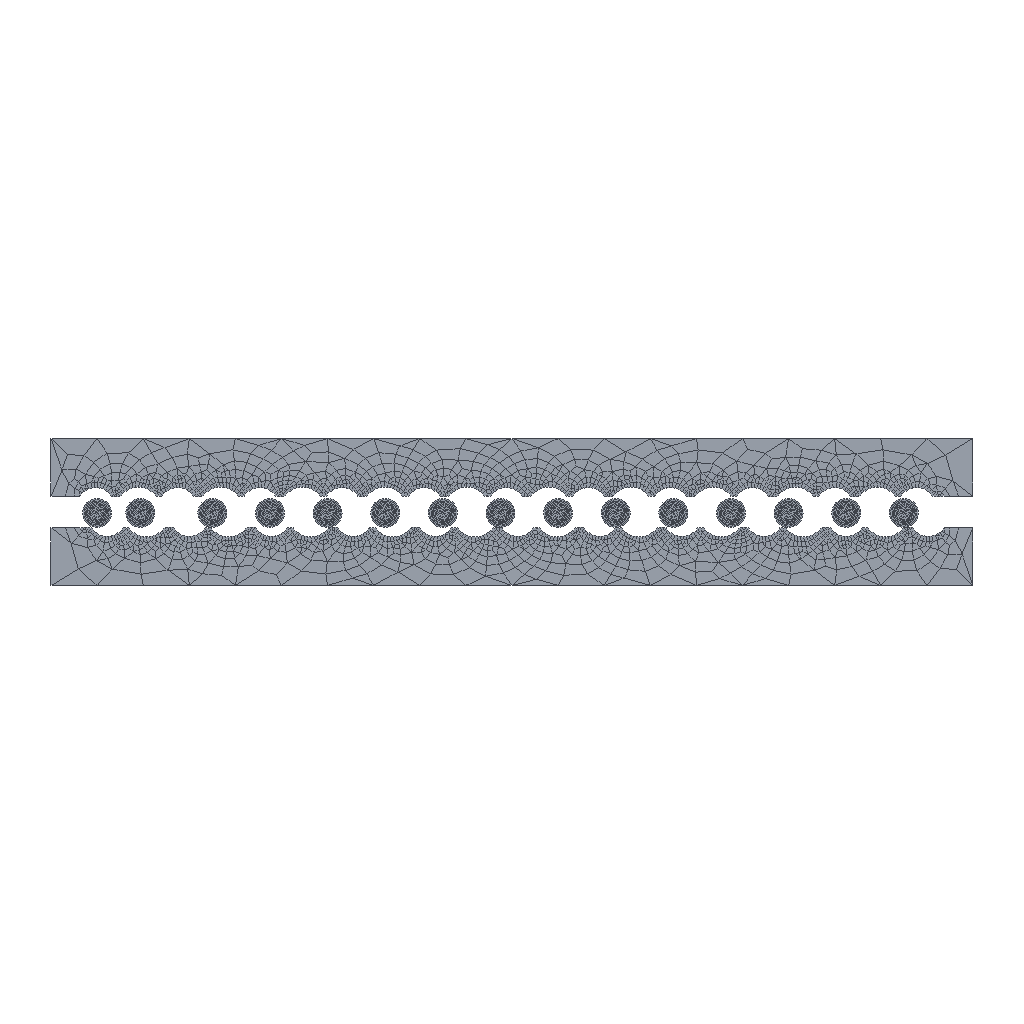Simulation study | abaqus
Set-up summary:
category,name,step,type,value,unit,region
solver,abaqus
solver,version,,,Abaqus/Explicit 2020
units,not stated in the deck,,not stated
analysis,deck,,transient,transient
load_step,Step-1,Step-1,transient
load_step,Step-2,Step-2,transient
load_step,requested,,,2
mesh,nodes,,,9465
mesh,elements,,,8789
element_type,CPS3,,plane,357
element_type,CPS4R,,plane,8432
load,load commands in deck,,count,2
bc,support commands in deck,,count,9
material,MATERIAL-1,,in results
material,MATERIAL-2,,in results
check,setup vs results,,match,"per instance, exact: element labels, types and connectivity; labels of the nodes the elements use; coordinates of those nodes at SINGLE_PRECISION in 16 of 17 instance(s)"
Abaqus input file, long lists of numbers shortened:
*Heading
** Job name: Job-1 Model name: Model-1
** Generated by: Abaqus/CAE 2020
*Preprint, echo=NO, model=NO, history=NO, contact=NO
**
** PARTS
**
*Part, name=sphere
*Node
      1,  0.4747, -0.1571
      2,  0.4964, -0.05996
** (459 more lines like these left out)
*Element, type=CPS3
 1, 422, 236, 213
 2, 233, 451, 245
** (11 more lines like these left out)
*Element, type=CPS4R
 14,  40,   9,  76, 129
 15,  77, 400,  10,  42
** (420 more lines like these left out)
*Nset, nset=Set-1, generate
   1,  461,    1
*Elset, elset=Set-1, generate
   1,  435,    1
** Section: Section-2
*Solid Section, elset=Set-1, material=Material-2
,
*End Part
**
*Part, name=up
*Node
      1,           0.,          -3.
      2,           0.,          -5.
** (1273 more lines like these left out)
*Element, type=CPS3
 1, 1033,    4,  148
 2,  376,  722, 1056
** (79 more lines like these left out)
*Element, type=CPS4R
  82,  418, 1034,  144,  145
  83, 1033,  454,  737,  374
** (1049 more lines like these left out)
*Nset, nset=Set-1, generate
    1,  1275,     1
*Elset, elset=Set-1, generate
    1,  1132,     1
** Section: Section-1
*Solid Section, elset=Set-1, material=Material-1
,
*End Part
**
**
** ASSEMBLY
**
*Assembly, name=Assembly
**
*Instance, name=sphere-1, part=sphere
         1.6,    -5.285,           0.
*End Instance
**
*Instance, name=up-1, part=up
          0.,          0.3,           0.
*End Instance
**
*Instance, name=sphere-1-lin-2-1, part=sphere
         3.1,    -5.285,           0.
*End Instance
**
*Instance, name=sphere-1-lin-3-1, part=sphere
         5.6,    -5.285,           0.
*End Instance
**
*Instance, name=sphere-1-lin-4-1, part=sphere
         7.6,    -5.285,           0.
*End Instance
**
*Instance, name=sphere-1-lin-5-1, part=sphere
         9.6,    -5.285,           0.
*End Instance
**
*Instance, name=sphere-1-lin-6-1, part=sphere
        11.6,    -5.285,           0.
*End Instance
**
*Instance, name=sphere-1-lin-7-1, part=sphere
        13.6,    -5.285,           0.
*End Instance
**
*Instance, name=sphere-1-lin-8-1, part=sphere
        15.6,    -5.285,           0.
*End Instance
**
*Instance, name=sphere-1-lin-9-1, part=sphere
        17.6,    -5.285,           0.
*End Instance
**
*Instance, name=sphere-1-lin-10-1, part=sphere
        19.6,    -5.285,           0.
*End Instance
**
*Instance, name=sphere-1-lin-11-1, part=sphere
        21.6,    -5.285,           0.
*End Instance
**
*Instance, name=sphere-1-lin-12-1, part=sphere
        23.6,    -5.285,           0.
*End Instance
**
*Instance, name=sphere-1-lin-13-1, part=sphere
        25.6,    -5.285,           0.
*End Instance
**
*Instance, name=sphere-1-lin-14-1, part=sphere
        27.6,    -5.285,           0.
*End Instance
**
*Instance, name=sphere-1-lin-15-1, part=sphere
        29.6,    -5.285,           0.
*End Instance
**
*Instance, name=up-3, part=up
         32.,        -10.8,           0.
         32.,        -10.8,           0.,          32.,        -10.8,           1.,         180.
*End Instance
**
*Node
      1,          16.,  -2.7,           0.
*Node
      2,          16.,  -7.8,           0.
*Nset, nset=Set-1, instance=up-3
   1, 132, 133, 134, 135, 136, 137, 138, 139, 140, 141, 142, 143, 358, 359, 360
 361, 362, 363, 364, 365
*Elset, elset=Set-1, instance=up-3
   44,   46,   47,   49,   50,   51,   61,   65,   67,   68,  979,  991, 1026, 1034, 1052, 1053
 1054, 1094, 1100, 1103
*Nset, nset=Set-2, instance=up-1
   1, 132, 133, 134, 135, 136, 137, 138, 139, 140, 141, 142, 143, 358, 359, 360
 361, 362, 363, 364, 365
*Elset, elset=Set-2, instance=up-1
   44,   46,   47,   49,   50,   51,   61,   65,   67,   68,  979,  991, 1026, 1034, 1052, 1053
 1054, 1094, 1100, 1103
*Nset, nset=Set-3, instance=up-3
   1, 132, 133, 134, 135, 136, 137, 138, 139, 140, 141, 142, 143, 358, 359, 360
 361, 362, 363, 364, 365
*Elset, elset=Set-3, instance=up-3
   44,   46,   47,   49,   50,   51,   61,   65,   67,   68,  979,  991, 1026, 1034, 1052, 1053
 1054, 1094, 1100, 1103
*Nset, nset=Set-6
 2,
*Nset, nset=Set-7
 1,
*Nset, nset=m_Set-4
 1,
*Nset, nset=m_Set-5
 2,
*Elset, elset=_Surf-1_S2, internal, instance=up-1
   44,   46,   47,   49,   50,   51,   61,   65,   67,   68, 1052, 1103
*Elset, elset=_Surf-1_S3, internal, instance=up-1
  979, 1053, 1094, 1100
*Elset, elset=_Surf-1_S4, internal, instance=up-1
  991, 1026
*Elset, elset=_Surf-1_S1, internal, instance=up-1
 1034, 1054
*Surface, type=ELEMENT, name=Surf-1
_Surf-1_S2, S2
_Surf-1_S3, S3
_Surf-1_S4, S4
_Surf-1_S1, S1
*Elset, elset=_s_Surf-2_S2, internal, instance=up-1
   44,   46,   47,   49,   50,   51,   61,   65,   67,   68, 1052, 1103
*Elset, elset=_s_Surf-2_S3, internal, instance=up-1
  979, 1053, 1094, 1100
*Elset, elset=_s_Surf-2_S4, internal, instance=up-1
  991, 1026
*Elset, elset=_s_Surf-2_S1, internal, instance=up-1
 1034, 1054
*Surface, type=ELEMENT, name=s_Surf-2
_s_Surf-2_S2, S2
_s_Surf-2_S3, S3
_s_Surf-2_S4, S4
_s_Surf-2_S1, S1
*Elset, elset=_s_Surf-3_S2, internal, instance=up-3
   44,   46,   47,   49,   50,   51,   61,   65,   67,   68, 1052, 1103
*Elset, elset=_s_Surf-3_S3, internal, instance=up-3
  979, 1053, 1094, 1100
*Elset, elset=_s_Surf-3_S4, internal, instance=up-3
  991, 1026
*Elset, elset=_s_Surf-3_S1, internal, instance=up-3
 1034, 1054
*Surface, type=ELEMENT, name=s_Surf-3
_s_Surf-3_S2, S2
_s_Surf-3_S3, S3
_s_Surf-3_S4, S4
_s_Surf-3_S1, S1
** Constraint: Constraint-1
*Coupling, constraint name=Constraint-1, ref node=m_Set-4, surface=s_Surf-2
*Kinematic
** Constraint: Constraint-2
*Coupling, constraint name=Constraint-2, ref node=m_Set-5, surface=s_Surf-3
*Kinematic
*End Assembly
*Amplitude, name=Amp-1
             0.,              0.,             0.1,              1.
**
** MATERIALS
**
*Material, name=Material-1
*Density
 2e-09,
*Elastic
1500., 0.35
*Plastic
100.,0.
*Material, name=Material-2
*Density
 2.5e-09,
*Elastic
1000., 0.32
**
** INTERACTION PROPERTIES
**
*Surface Interaction, name=IntProp-1
*Friction
 0.2,
*Surface Behavior, pressure-overclosure=HARD
**
** INTERACTIONS
**
** Interaction: Int-1
*Contact, op=NEW
*Contact Inclusions, ALL EXTERIOR
*Contact Property Assignment
 ,  , IntProp-1
** ----------------------------------------------------------------
**
** STEP: Step-1
**
*Step, name=Step-1, nlgeom=YES
*Dynamic, Explicit
, 0.1
*Bulk Viscosity
0.06, 1.2
** Mass Scaling: Semi-Automatic
**               Whole Model
*Fixed Mass Scaling, factor=500.
**
** BOUNDARY CONDITIONS
**
** Name: BC-2 Type: 位移/转角
*Boundary
Set-7, 1, 1
Set-7, 6, 6
** Name: [REDACTED] : Displacement/rotation angle
*Boundary
Set-6, 1, 1
Set-6, 2, 2
Set-6, 6, 6
**
** LOADS
**
** Name: Load-1   Type: Pressure
*Dsload
Surf-1, P, 0.1
**
** OUTPUT REQUESTS
**
*Restart, write, number interval=1, time marks=NO
**
** FIELD OUTPUT: F-Output-1
**
*Output, field, number interval=50
*Node Output
A, CF, RF, RM, RT, U, V
*Element Output, directions=YES
E, EVF, LE, MISES, MISESMAX, PE, PEEQ, PEEQVAVG, PEVAVG, S, SF, SVAVG, YIELDPOT
*Contact Output
CDISP, CSTRESS
*Output, history, frequency=0
*End Step
** ----------------------------------------------------------------
**
** STEP: Step-2
**
*Step, name=Step-2, nlgeom=YES
*Dynamic, Explicit
, 0.1
*Bulk Viscosity
0.06, 1.2
** Mass Scaling: Semi-Automatic
**               Whole Model
*Fixed Mass Scaling, factor=500.
**
** BOUNDARY CONDITIONS
**
** Name: BC-2 Type: 位移/转角
*Boundary
Set-7, 2, 2
** Name: [REDACTED] : Displacement/rotation angle
*Boundary, amplitude=Amp-1
Set-6, 1, 1, -2.
Set-6, 2, 2
Set-6, 6, 6
**
** OUTPUT REQUESTS
**
*Restart, write, number interval=1, time marks=NO
**
** FIELD OUTPUT: F-Output-1
**
*Output, field, number interval=50
*Node Output
A, CF, RF, RM, RT, U, V
*Element Output, directions=YES
E, EVF, LE, MISES, MISESMAX, PE, PEEQ, PEEQVAVG, PEVAVG, S, SF, SVAVG, YIELDPOT
*Contact Output
CDISP, CSTRESS
**
** HISTORY OUTPUT: H-Output-2
**
*Output, history, time interval=1e-05
*Node Output, nset=Set-6
RF1, RF2
**
** HISTORY OUTPUT: H-Output-1
**
*Contact Output, surface=Surf-1
CFS1, CFS2, CFS3, CFSM, CFT1, CFT2, CFT3, CFTM
*End Step
Results summary:
result,step,Step-1,completed,increments=132849 time=0.1/0.1
result,step,Step-2,completed,increments=132867 time=0.1/0.1
result,analysis,,,transient
result,last_loadstep,,,2
result,primary field,,,U
result,reaction total,,FX,2.916,model units
result,reaction total,,FY,3.257,model units
result,reaction total,,FZ,0.0,model units